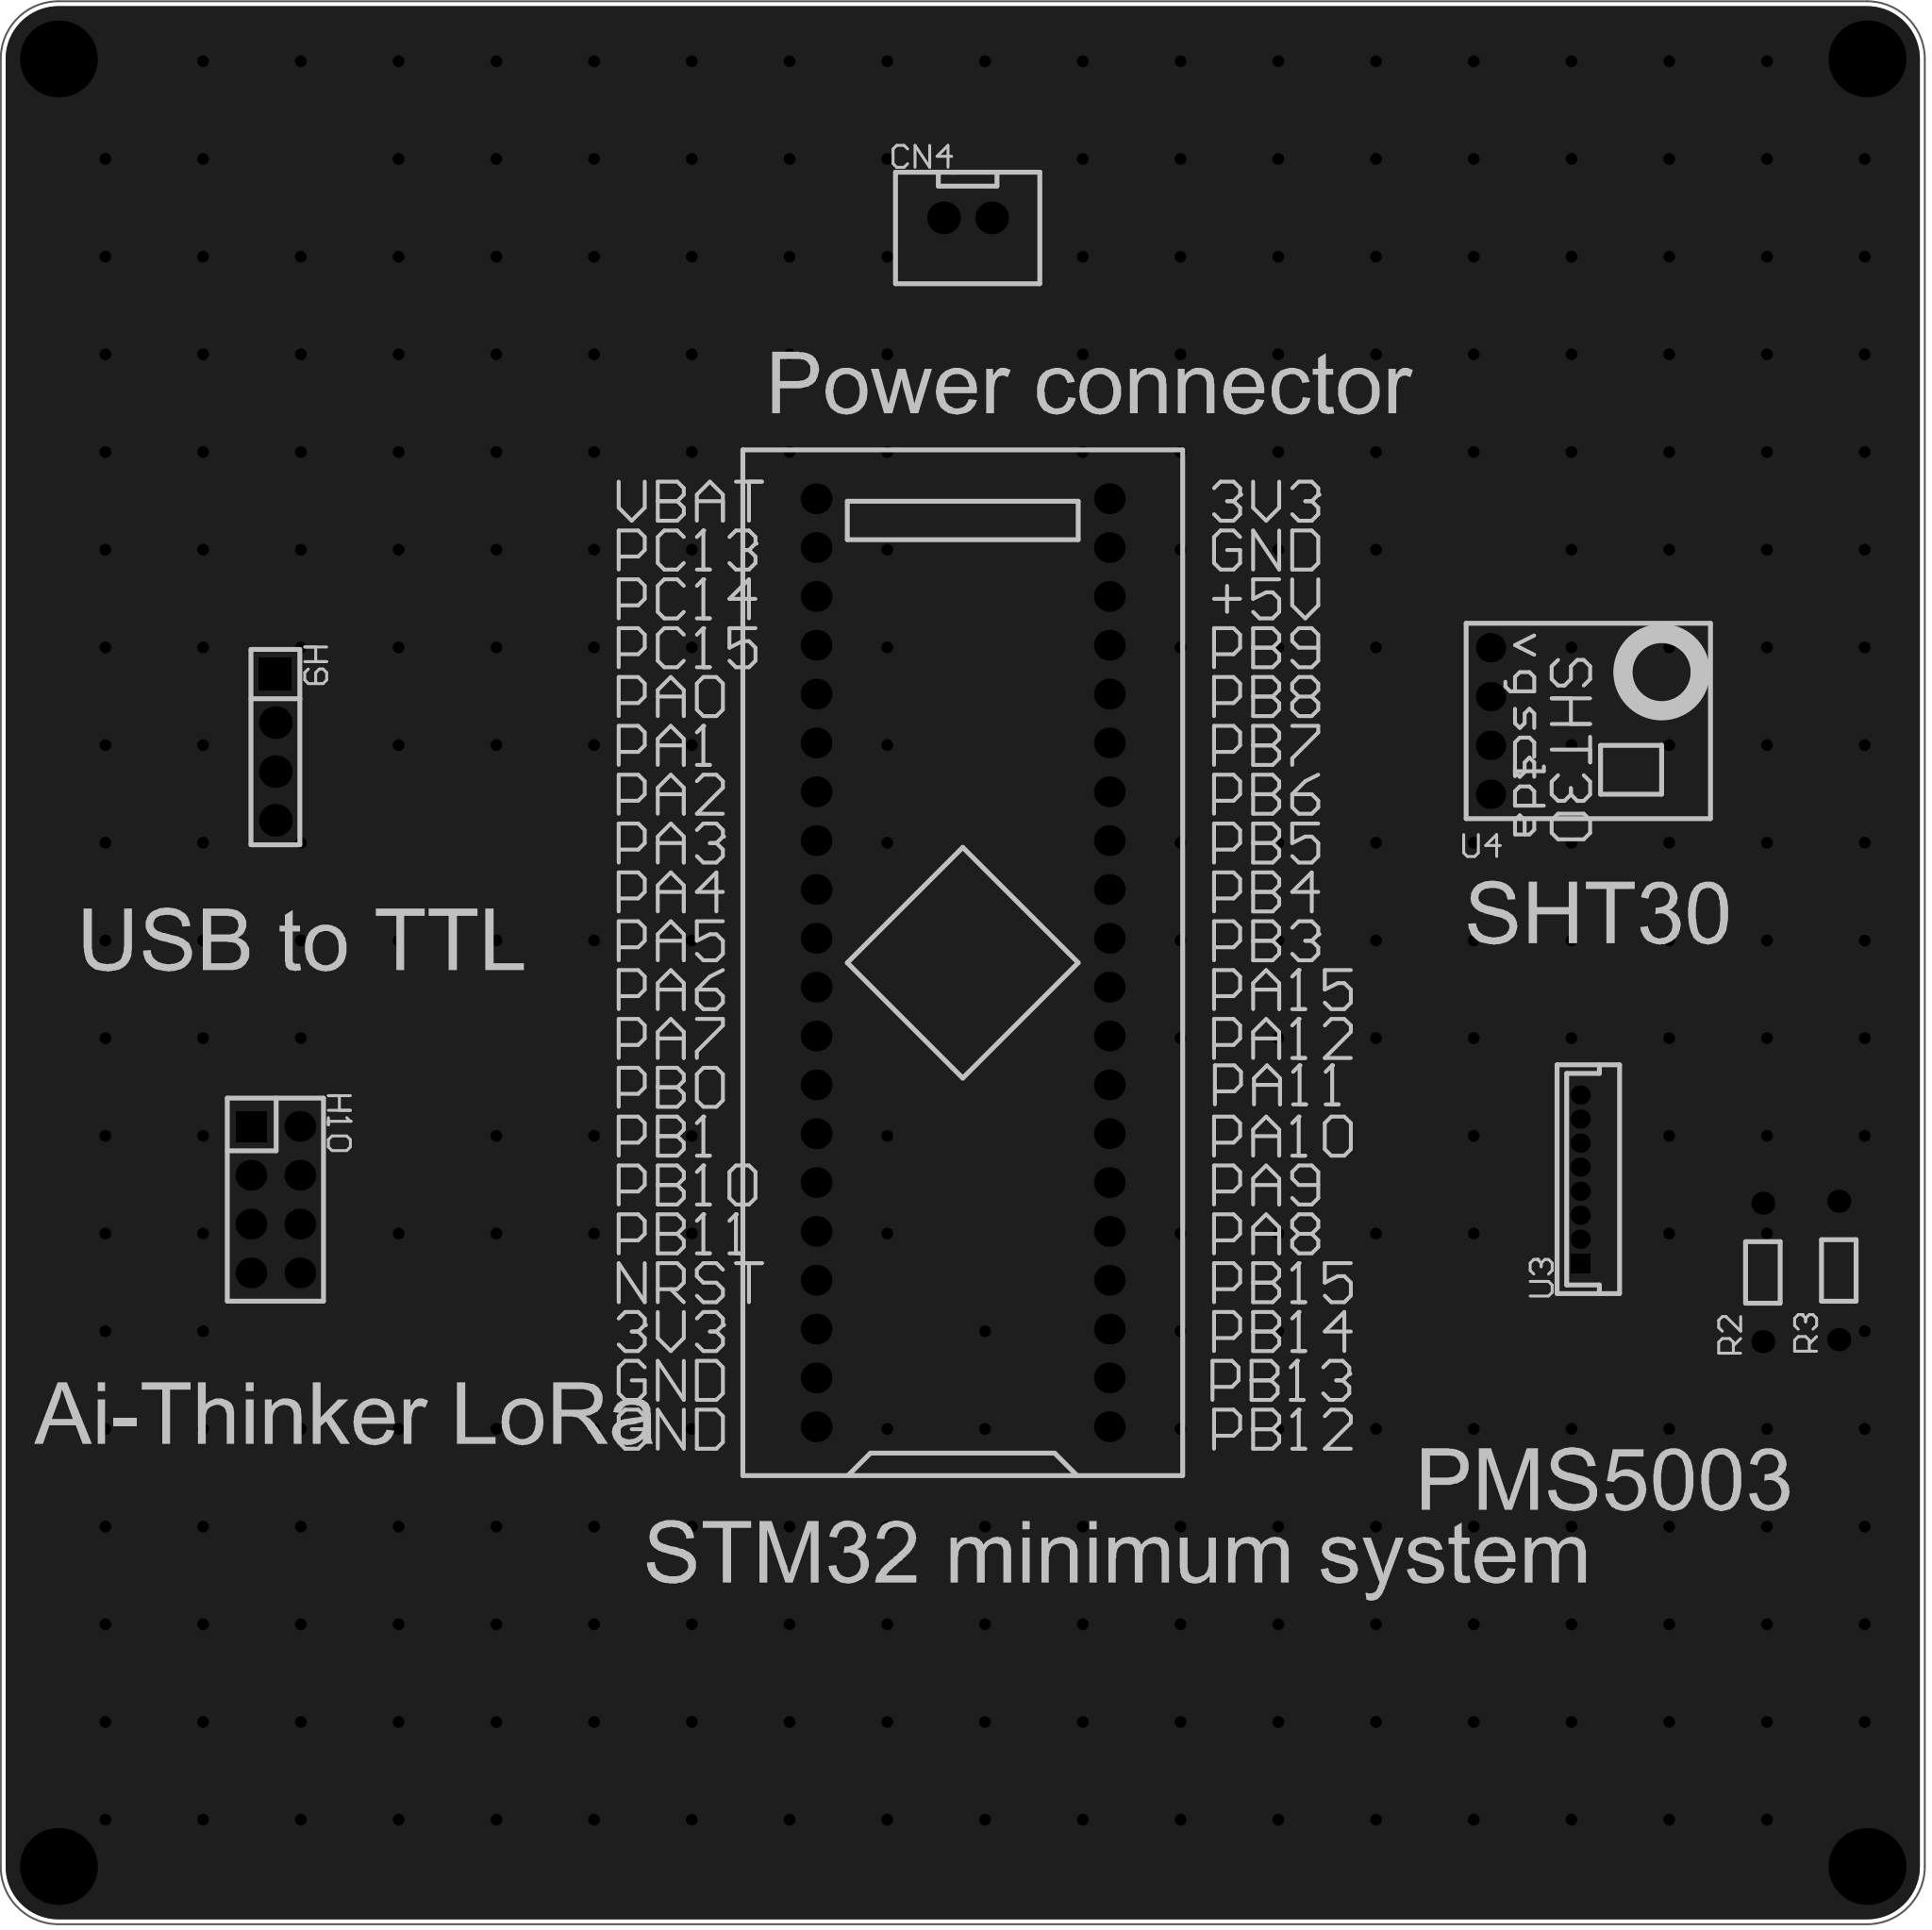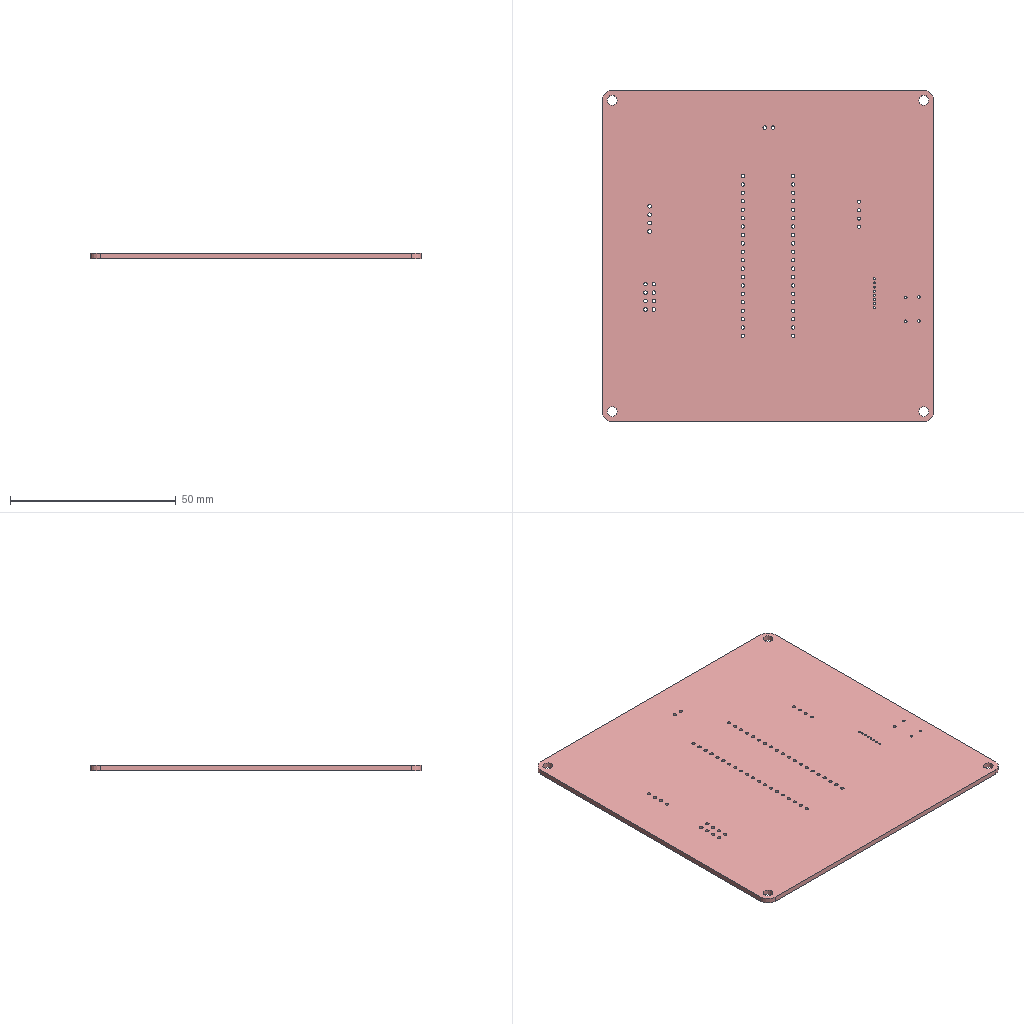Circuit board layout | Altium Designer | box 100 x 100 x 1.6 mm
Layer stack:
# Altium Designer layer stack of  (unit mm; dielectric type: 0 none, 1 core, 2 prepreg, 3 surface material)
index,name,kind,layer,copper_thickness_mm,dielectric_type,dielectric_thickness_mm,dielectric_material,dielectric_constant
0,Top Paste Mask Layer,other,,,,,,
1,Top Silkscreen Layer,other,,,,,,
2,Top Solder Mask Layer,dielectric,,,3,0.01,,3.3
3,Top Layer,copper,Top Layer,0.035,,,,
4,Dielectric1,dielectric,,,3,1.51,FR4,4.5
5,Bottom Layer,copper,Bottom Layer,0.035,,,,
6,Bottom Solder Mask Layer,dielectric,,,3,0.01,,3.3
7,Bottom Silkscreen Layer,other,,,,,,
8,Bottom Paste Mask Layer,other,,,,,,
# drill layer pairs: low layer,high layer
drill_pair,Top Layer,Bottom Layer
Part placement:
Designator,Comment,Layer,Footprint,Center-X(mm),Center-Y(mm),Rotation
U1,STM32F103C8T6-Card,TopLayer,CONN-TH_L53.3-W22.9_STM32F103C8T6-CARD,141.351,130.937,90
CN4,XH2.54*2P_THT,TopLayer,CONN-TH_2P-P2.50-XH2.54-2P,141.605,169.672,0
H9,,TopLayer,HDR-TH_4P-P2.54-V-M,105.626,142.15,270
H10,,TopLayer,HDR-TH_8P-P2.54-V-F-R2-C4-S2.54-1,105.626,118.618,270
R2,1kΩ,TopLayer,Res_1/8W,182.935,114.832,90
R3,10kΩ,TopLayer,Res_1/8W,186.881,114.935,90
U3,PMS5003,TopLayer,1.25-LI-8P,173.438,119.681,90
U4,,TopLayer,SHT30模块,168.783,143.51,0
Pad and via stacks:
# Altium Designer via and pad stacks of  (unit mm). Each distinct definition once, with the count of objects using it.
# via: kind,start_layer,end_layer,hole_mm,diameter_mm,mode(0 simple;1 top-mid-bottom;2 full stack),diameter_per_layer,count,example_net
# pad: kind,layer,hole_mm,hole_type(0 round;1 square;2 slot),plating,top_size,top_shape(1 round;2 rect;3 octagon;9 rounded rect),mid_size,bottom_size,mode,footprint,size_per_layer,count,example
pad,Multi-Layer,3,0,plated,4x4,1,4x4,4x4,0,,,4,1
pad,Multi-Layer,1,0,plated,1.6x1.6,1,1.6x1.6,1.6x1.6,0,CONN-TH_L53.3-W22.9_STM32F103C8T6-CARD,,40,U1.1
pad,Multi-Layer,1.05,0,plated,1.7x1.7,1,1.7x1.7,1.7x1.7,0,CONN-TH_2P-P2.50-XH2.54-2P,,2,CN4.2
pad,Multi-Layer,1.1,0,plated,1.7x1.7,2,1.7x1.7,1.7x1.7,0,HDR-TH_4P-P2.54-V-M,,1,H9.1
pad,Multi-Layer,1.1,0,plated,1.7x1.7,1,1.7x1.7,1.7x1.7,0,HDR-TH_4P-P2.54-V-M,,3,H9.2
pad,Multi-Layer,1.1,0,plated,1.6x1.6,2,1.6x1.6,1.6x1.6,0,HDR-TH_8P-P2.54-V-F-R2-C4-S2.54-1,,1,H10.1
pad,Multi-Layer,1.1,0,plated,1.6x1.6,1,1.6x1.6,1.6x1.6,0,HDR-TH_8P-P2.54-V-F-R2-C4-S2.54-1,,7,H10.2
pad,Multi-Layer,0.8001,0,plated,1.199x1.199,1,1.199x1.199,1.199x1.199,0,Res_1/8W,,4,R2.1
pad,Multi-Layer,0.6,0,plated,1x1,1,1x1,1x1,0,1.25-LI-8P,,7,U3.8
pad,Multi-Layer,0.6,0,plated,1x1,2,1x1,1x1,0,1.25-LI-8P,,1,U3.1
pad,Multi-Layer,0.9144,0,plated,1.524x1.524,1,1.524x1.524,1.524x1.524,0,SHT30\u00C4\u00A3\u00BF\u00E9,,4,U4.4
via,Top Layer,Bottom Layer,0.3048,0.61,0,,288,GND
Copper pours:
name,layer,net,type(0 solid;1 hatched;2 none)
Bottom Layer-GND,Bottom Layer,GND,0
Top Layer-GND,Top Layer,GND,0
Design rules, without the lines most boards share:
# Altium Designer design rules of  (exported by Altium Designer, unit mm)
# columns: name | kind | enabled | priority | scope1 | scope2 | descriptor | typed fields (field=value)
Copper_copperRegion_copperThickness1oz | 0 | disabled | 4 | All | All | Clearance Constraint (Gap=5.984mil) (Disabled)(All),(All) | gap=0.152
Copper_copperRegion_copperThickness1oz_1 | 63 | disabled | 4 | All | All | Board Clearance Constraint (Gap=0mil) (Disabled)(All) |
Copper_copperRegion_Copper_copperRegion | 0 | disabled | 5 | All | All | Clearance Constraint (Gap=5.984mil) (Disabled)(All),(All) | gap=0.152
Copper_copperRegion_Copper_copperRegion_1 | 63 | disabled | 5 | All | All | Board Clearance Constraint (Gap=0mil) (Disabled)(All) |
copperThickness1oz | 0 | enabled | 6 | All | All | Clearance Constraint (Gap=5.984mil) (All),(All) | gap=0.152
copperThickness1oz_1 | 63 | enabled | 6 | All | All | Board Clearance Constraint (Gap=0mil) (All) |
copperRegion_copperThickness1oz | 20 | disabled | 1 | All | All | Polygon Connect Rule(Relief Connect )(Conductor Width=10mil) (Relief Angle=90 Angle) (Entries=4) (Air Gap Width=10mil) (Disabled)(All),(All) | connect_style(0=relief,1=direct,2=none)=0 relief_conductor_width=0.254 relief_entries=4
copperRegion_Copper_copperRegion | 20 | disabled | 2 | All | All | Polygon Connect Rule(Relief Connect )(Conductor Width=10mil) (Relief Angle=90 Angle) (Entries=4) (Air Gap Width=10mil) (Disabled)(All),(All) | connect_style(0=relief,1=direct,2=none)=0 relief_conductor_width=0.254 relief_entries=4
copperRegion | 20 | enabled | 3 | All | All | Polygon Connect Rule(Relief Connect )(Conductor Width=10mil) (Relief Angle=90 Angle) (Entries=4) (Air Gap Width=10mil) (All),(All) | connect_style(0=relief,1=direct,2=none)=0 relief_conductor_width=0.254 relief_entries=4